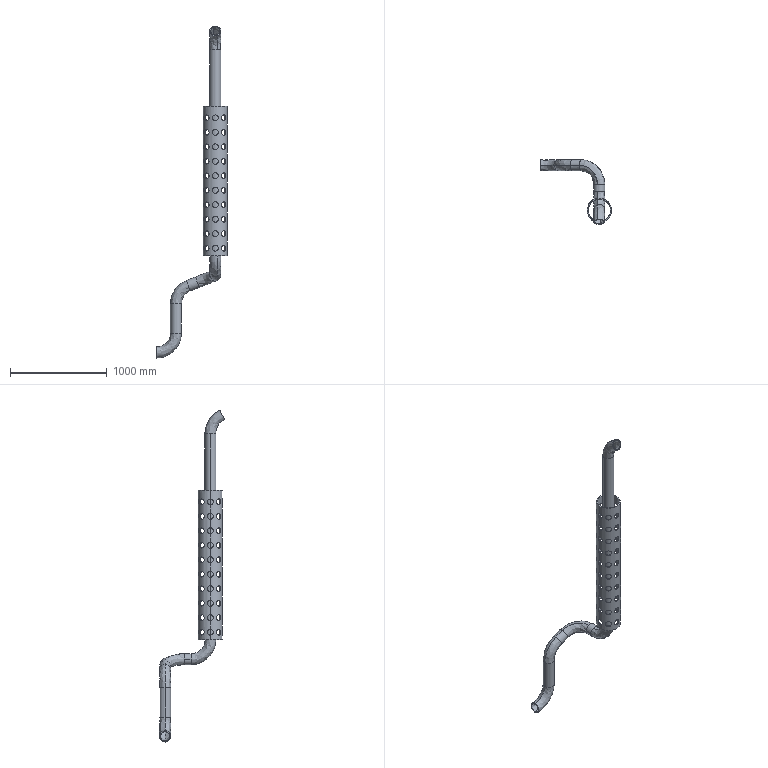Part | STEP file | echap-3 | 2 solids | 204 faces | box 732.765 x 673.421 x 3439 mm | volume 22710287 mm3 | cylinder 180 | spline 20 | plane 4 | commonest cylinder face diameters 60 x160 95 x8 115 x8 230 x2 250 x2